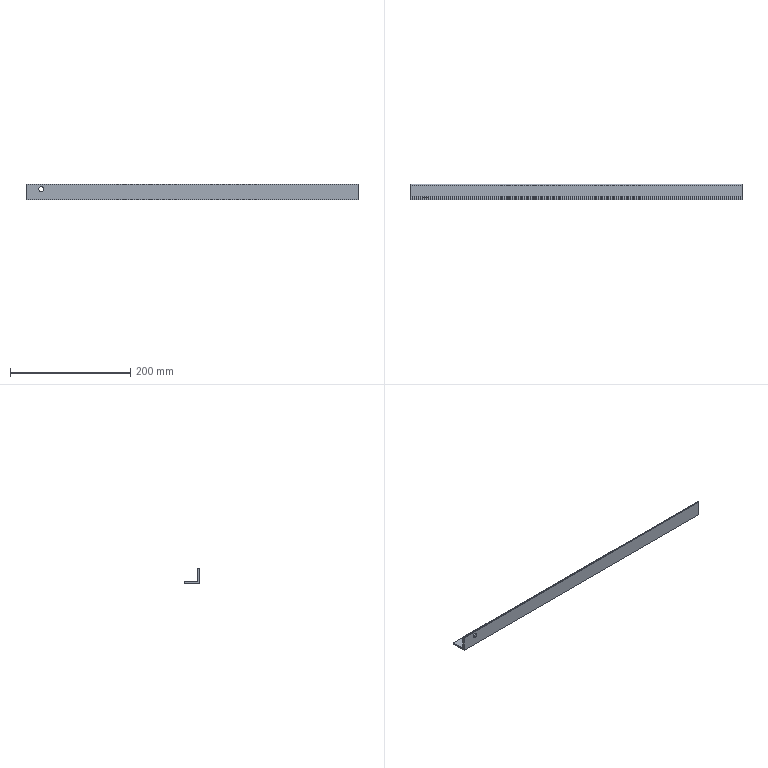Part | NX | features BREP 1 | 1 solid | 13 faces | box 552.45 x 25.4 x 25.4 mm | volume 83062 mm3 | plane 8 | cylinder 5 | commonest cylinder face diameters 3.175 x3 8.382 x2
STEP:
#1=CARTESIAN_POINT('',(-276.225,1.587,25.4));
#2=VERTEX_POINT('',#1);
#3=CARTESIAN_POINT('',(-276.225,3.175,23.812));
#4=VERTEX_POINT('',#3);
#5=CARTESIAN_POINT('',(-276.225,1.587,23.812));
#6=DIRECTION('',(-1.,0.,0.));
#7=DIRECTION('',(0.,0.,1.));
#8=AXIS2_PLACEMENT_3D('',#5,#6,#7);
#9=CIRCLE('',#8,1.587);
#10=EDGE_CURVE('',#2,#4,#9,.T.);
#11=ORIENTED_EDGE('',*,*,#10,.T.);
#12=CARTESIAN_POINT('',(-276.225,3.175,4.763));
#13=VERTEX_POINT('',#12);
#14=CARTESIAN_POINT('',(-276.225,3.175,4.763));
#15=DIRECTION('',(0.,0.,1.));
#16=VECTOR('',#15,1000.);
#17=LINE('',#14,#16);
#18=EDGE_CURVE('',#13,#4,#17,.T.);
#19=ORIENTED_EDGE('',*,*,#18,.F.);
#20=CARTESIAN_POINT('',(-276.225,4.763,3.175));
#21=VERTEX_POINT('',#20);
#22=CARTESIAN_POINT('',(-276.225,4.763,4.763));
#23=DIRECTION('',(1.,0.,0.));
#24=DIRECTION('',(0.,-1.,0.));
#25=AXIS2_PLACEMENT_3D('',#22,#23,#24);
#26=CIRCLE('',#25,1.587);
#27=EDGE_CURVE('',#13,#21,#26,.T.);
#28=ORIENTED_EDGE('',*,*,#27,.T.);
#29=CARTESIAN_POINT('',(-276.225,23.812,3.175));
#30=VERTEX_POINT('',#29);
#31=CARTESIAN_POINT('',(-276.225,23.812,3.175));
#32=DIRECTION('',(0.,-1.,0.));
#33=VECTOR('',#32,1000.);
#34=LINE('',#31,#33);
#35=EDGE_CURVE('',#30,#21,#34,.T.);
#36=ORIENTED_EDGE('',*,*,#35,.F.);
#37=CARTESIAN_POINT('',(-276.225,25.4,1.587));
#38=VERTEX_POINT('',#37);
#39=CARTESIAN_POINT('',(-276.225,23.812,1.587));
#40=DIRECTION('',(-1.,0.,0.));
#41=DIRECTION('',(0.,0.,1.));
#42=AXIS2_PLACEMENT_3D('',#39,#40,#41);
#43=CIRCLE('',#42,1.587);
#44=EDGE_CURVE('',#30,#38,#43,.T.);
#45=ORIENTED_EDGE('',*,*,#44,.T.);
#46=CARTESIAN_POINT('',(-276.225,25.4,0.));
#47=VERTEX_POINT('',#46);
#48=CARTESIAN_POINT('',(-276.225,25.4,0.));
#49=DIRECTION('',(0.,0.,1.));
#50=VECTOR('',#49,1000.);
#51=LINE('',#48,#50);
#52=EDGE_CURVE('',#47,#38,#51,.T.);
#53=ORIENTED_EDGE('',*,*,#52,.F.);
#54=CARTESIAN_POINT('',(-276.225,0.,0.));
#55=VERTEX_POINT('',#54);
#56=CARTESIAN_POINT('',(-276.225,0.,0.));
#57=DIRECTION('',(0.,1.,0.));
#58=VECTOR('',#57,1000.);
#59=LINE('',#56,#58);
#60=EDGE_CURVE('',#55,#47,#59,.T.);
#61=ORIENTED_EDGE('',*,*,#60,.F.);
#62=CARTESIAN_POINT('',(-276.225,0.,25.4));
#63=VERTEX_POINT('',#62);
#64=CARTESIAN_POINT('',(-276.225,0.,25.4));
#65=DIRECTION('',(0.,0.,-1.));
#66=VECTOR('',#65,1000.);
#67=LINE('',#64,#66);
#68=EDGE_CURVE('',#63,#55,#67,.T.);
#69=ORIENTED_EDGE('',*,*,#68,.F.);
#70=CARTESIAN_POINT('',(-276.225,1.587,25.4));
#71=DIRECTION('',(0.,-1.,0.));
#72=VECTOR('',#71,1000.);
#73=LINE('',#70,#72);
#74=EDGE_CURVE('',#2,#63,#73,.T.);
#75=ORIENTED_EDGE('',*,*,#74,.F.);
#76=EDGE_LOOP('',(#11,#19,#28,#36,#45,#53,#61,#69,#75));
#77=FACE_BOUND('',#76,.T.);
#78=CARTESIAN_POINT('',(-276.225,0.,0.));
#79=DIRECTION('',(1.,0.,0.));
#80=DIRECTION('',(0.,1.,0.));
#81=AXIS2_PLACEMENT_3D('',#78,#79,#80);
#82=PLANE('',#81);
#83=ADVANCED_FACE('',(#77),#82,.F.);
#84=CARTESIAN_POINT('',(276.225,0.,25.4));
#85=VERTEX_POINT('',#84);
#86=CARTESIAN_POINT('',(-276.225,0.,25.4));
#87=DIRECTION('',(1.,0.,0.));
#88=VECTOR('',#87,1000.);
#89=LINE('',#86,#88);
#90=EDGE_CURVE('',#63,#85,#89,.T.);
#91=ORIENTED_EDGE('',*,*,#90,.T.);
#92=CARTESIAN_POINT('',(276.225,1.587,25.4));
#93=VERTEX_POINT('',#92);
#94=CARTESIAN_POINT('',(276.225,1.587,25.4));
#95=DIRECTION('',(0.,-1.,0.));
#96=VECTOR('',#95,1000.);
#97=LINE('',#94,#96);
#98=EDGE_CURVE('',#93,#85,#97,.T.);
#99=ORIENTED_EDGE('',*,*,#98,.F.);
#100=CARTESIAN_POINT('',(276.225,1.587,25.4));
#101=DIRECTION('',(-1.,0.,0.));
#102=VECTOR('',#101,1000.);
#103=LINE('',#100,#102);
#104=EDGE_CURVE('',#93,#2,#103,.T.);
#105=ORIENTED_EDGE('',*,*,#104,.T.);
#106=ORIENTED_EDGE('',*,*,#74,.T.);
#107=EDGE_LOOP('',(#91,#99,#105,#106));
#108=FACE_BOUND('',#107,.T.);
#109=CARTESIAN_POINT('',(-276.225,3.175,25.4));
#110=DIRECTION('',(0.,0.,1.));
#111=DIRECTION('',(1.,0.,0.));
#112=AXIS2_PLACEMENT_3D('',#109,#110,#111);
#113=PLANE('',#112);
#114=ADVANCED_FACE('',(#108),#113,.T.);
#115=CARTESIAN_POINT('',(276.225,3.175,23.812));
#116=VERTEX_POINT('',#115);
#117=CARTESIAN_POINT('',(276.225,1.587,23.812));
#118=DIRECTION('',(1.,0.,0.));
#119=DIRECTION('',(0.,1.,0.));
#120=AXIS2_PLACEMENT_3D('',#117,#118,#119);
#121=CIRCLE('',#120,1.587);
#122=EDGE_CURVE('',#116,#93,#121,.T.);
#123=ORIENTED_EDGE('',*,*,#122,.F.);
#124=CARTESIAN_POINT('',(276.225,3.175,23.812));
#125=DIRECTION('',(-1.,0.,0.));
#126=VECTOR('',#125,1000.);
#127=LINE('',#124,#126);
#128=EDGE_CURVE('',#116,#4,#127,.T.);
#129=ORIENTED_EDGE('',*,*,#128,.T.);
#130=ORIENTED_EDGE('',*,*,#10,.F.);
#131=ORIENTED_EDGE('',*,*,#104,.F.);
#132=EDGE_LOOP('',(#123,#129,#130,#131));
#133=FACE_BOUND('',#132,.T.);
#134=CARTESIAN_POINT('',(277.091,1.587,23.812));
#135=DIRECTION('',(-1.,0.,0.));
#136=DIRECTION('',(0.,0.,1.));
#137=AXIS2_PLACEMENT_3D('',#134,#135,#136);
#138=CYLINDRICAL_SURFACE('',#137,1.587);
#139=ADVANCED_FACE('',(#133),#138,.T.);
#140=CARTESIAN_POINT('',(276.225,3.175,4.763));
#141=VERTEX_POINT('',#140);
#142=CARTESIAN_POINT('',(276.225,3.175,4.763));
#143=DIRECTION('',(0.,0.,1.));
#144=VECTOR('',#143,1000.);
#145=LINE('',#142,#144);
#146=EDGE_CURVE('',#141,#116,#145,.T.);
#147=ORIENTED_EDGE('',*,*,#146,.F.);
#148=CARTESIAN_POINT('',(-276.225,3.175,4.763));
#149=DIRECTION('',(1.,0.,0.));
#150=VECTOR('',#149,1000.);
#151=LINE('',#148,#150);
#152=EDGE_CURVE('',#13,#141,#151,.T.);
#153=ORIENTED_EDGE('',*,*,#152,.F.);
#154=ORIENTED_EDGE('',*,*,#18,.T.);
#155=ORIENTED_EDGE('',*,*,#128,.F.);
#156=EDGE_LOOP('',(#147,#153,#154,#155));
#157=FACE_BOUND('',#156,.T.);
#158=CARTESIAN_POINT('',(-255.016,3.175,17.475));
#159=VERTEX_POINT('',#158);
#160=CARTESIAN_POINT('',(-246.634,3.175,17.475));
#161=VERTEX_POINT('',#160);
#162=CARTESIAN_POINT('',(-250.825,3.175,17.475));
#163=DIRECTION('',(0.,-1.,0.));
#164=DIRECTION('',(-1.,0.,0.));
#165=AXIS2_PLACEMENT_3D('',#162,#163,#164);
#166=CIRCLE('',#165,4.191);
#167=EDGE_CURVE('',#159,#161,#166,.T.);
#168=ORIENTED_EDGE('',*,*,#167,.T.);
#169=CARTESIAN_POINT('',(-250.825,3.175,17.475));
#170=DIRECTION('',(0.,-1.,0.));
#171=DIRECTION('',(1.,0.,0.));
#172=AXIS2_PLACEMENT_3D('',#169,#170,#171);
#173=CIRCLE('',#172,4.191);
#174=EDGE_CURVE('',#161,#159,#173,.T.);
#175=ORIENTED_EDGE('',*,*,#174,.T.);
#176=EDGE_LOOP('',(#168,#175));
#177=FACE_BOUND('',#176,.T.);
#178=CARTESIAN_POINT('',(-276.225,3.175,3.175));
#179=DIRECTION('',(0.,1.,0.));
#180=DIRECTION('',(1.,0.,0.));
#181=AXIS2_PLACEMENT_3D('',#178,#179,#180);
#182=PLANE('',#181);
#183=ADVANCED_FACE('',(#157,#177),#182,.T.);
#184=CARTESIAN_POINT('',(276.225,4.763,3.175));
#185=VERTEX_POINT('',#184);
#186=CARTESIAN_POINT('',(276.225,4.763,4.763));
#187=DIRECTION('',(-1.,0.,0.));
#188=DIRECTION('',(0.,0.,-1.));
#189=AXIS2_PLACEMENT_3D('',#186,#187,#188);
#190=CIRCLE('',#189,1.587);
#191=EDGE_CURVE('',#185,#141,#190,.T.);
#192=ORIENTED_EDGE('',*,*,#191,.F.);
#193=CARTESIAN_POINT('',(-276.225,4.763,3.175));
#194=DIRECTION('',(1.,0.,0.));
#195=VECTOR('',#194,1000.);
#196=LINE('',#193,#195);
#197=EDGE_CURVE('',#21,#185,#196,.T.);
#198=ORIENTED_EDGE('',*,*,#197,.F.);
#199=ORIENTED_EDGE('',*,*,#27,.F.);
#200=ORIENTED_EDGE('',*,*,#152,.T.);
#201=EDGE_LOOP('',(#192,#198,#199,#200));
#202=FACE_BOUND('',#201,.T.);
#203=CARTESIAN_POINT('',(-276.965,4.763,4.763));
#204=DIRECTION('',(1.,0.,0.));
#205=DIRECTION('',(0.,-1.,0.));
#206=AXIS2_PLACEMENT_3D('',#203,#204,#205);
#207=CYLINDRICAL_SURFACE('',#206,1.587);
#208=ADVANCED_FACE('',(#202),#207,.F.);
#209=ORIENTED_EDGE('',*,*,#35,.T.);
#210=ORIENTED_EDGE('',*,*,#197,.T.);
#211=CARTESIAN_POINT('',(276.225,23.812,3.175));
#212=VERTEX_POINT('',#211);
#213=CARTESIAN_POINT('',(276.225,23.812,3.175));
#214=DIRECTION('',(0.,-1.,0.));
#215=VECTOR('',#214,1000.);
#216=LINE('',#213,#215);
#217=EDGE_CURVE('',#212,#185,#216,.T.);
#218=ORIENTED_EDGE('',*,*,#217,.F.);
#219=CARTESIAN_POINT('',(276.225,23.812,3.175));
#220=DIRECTION('',(-1.,0.,0.));
#221=VECTOR('',#220,1000.);
#222=LINE('',#219,#221);
#223=EDGE_CURVE('',#212,#30,#222,.T.);
#224=ORIENTED_EDGE('',*,*,#223,.T.);
#225=EDGE_LOOP('',(#209,#210,#218,#224));
#226=FACE_BOUND('',#225,.T.);
#227=CARTESIAN_POINT('',(-276.225,25.4,3.175));
#228=DIRECTION('',(0.,0.,1.));
#229=DIRECTION('',(1.,0.,0.));
#230=AXIS2_PLACEMENT_3D('',#227,#228,#229);
#231=PLANE('',#230);
#232=ADVANCED_FACE('',(#226),#231,.T.);
#233=CARTESIAN_POINT('',(276.225,25.4,1.587));
#234=VERTEX_POINT('',#233);
#235=CARTESIAN_POINT('',(276.225,23.812,1.587));
#236=DIRECTION('',(1.,0.,0.));
#237=DIRECTION('',(0.,1.,0.));
#238=AXIS2_PLACEMENT_3D('',#235,#236,#237);
#239=CIRCLE('',#238,1.587);
#240=EDGE_CURVE('',#234,#212,#239,.T.);
#241=ORIENTED_EDGE('',*,*,#240,.F.);
#242=CARTESIAN_POINT('',(276.225,25.4,1.587));
#243=DIRECTION('',(-1.,0.,0.));
#244=VECTOR('',#243,1000.);
#245=LINE('',#242,#244);
#246=EDGE_CURVE('',#234,#38,#245,.T.);
#247=ORIENTED_EDGE('',*,*,#246,.T.);
#248=ORIENTED_EDGE('',*,*,#44,.F.);
#249=ORIENTED_EDGE('',*,*,#223,.F.);
#250=EDGE_LOOP('',(#241,#247,#248,#249));
#251=FACE_BOUND('',#250,.T.);
#252=CARTESIAN_POINT('',(277.091,23.812,1.587));
#253=DIRECTION('',(-1.,0.,0.));
#254=DIRECTION('',(0.,0.,1.));
#255=AXIS2_PLACEMENT_3D('',#252,#253,#254);
#256=CYLINDRICAL_SURFACE('',#255,1.587);
#257=ADVANCED_FACE('',(#251),#256,.T.);
#258=ORIENTED_EDGE('',*,*,#246,.F.);
#259=CARTESIAN_POINT('',(276.225,25.4,0.));
#260=VERTEX_POINT('',#259);
#261=CARTESIAN_POINT('',(276.225,25.4,0.));
#262=DIRECTION('',(0.,0.,1.));
#263=VECTOR('',#262,1000.);
#264=LINE('',#261,#263);
#265=EDGE_CURVE('',#260,#234,#264,.T.);
#266=ORIENTED_EDGE('',*,*,#265,.F.);
#267=CARTESIAN_POINT('',(-276.225,25.4,0.));
#268=DIRECTION('',(1.,0.,0.));
#269=VECTOR('',#268,1000.);
#270=LINE('',#267,#269);
#271=EDGE_CURVE('',#47,#260,#270,.T.);
#272=ORIENTED_EDGE('',*,*,#271,.F.);
#273=ORIENTED_EDGE('',*,*,#52,.T.);
#274=EDGE_LOOP('',(#258,#266,#272,#273));
#275=FACE_BOUND('',#274,.T.);
#276=CARTESIAN_POINT('',(-276.225,25.4,0.));
#277=DIRECTION('',(0.,1.,0.));
#278=DIRECTION('',(1.,0.,0.));
#279=AXIS2_PLACEMENT_3D('',#276,#277,#278);
#280=PLANE('',#279);
#281=ADVANCED_FACE('',(#275),#280,.T.);
#282=ORIENTED_EDGE('',*,*,#271,.T.);
#283=CARTESIAN_POINT('',(276.225,0.,0.));
#284=VERTEX_POINT('',#283);
#285=CARTESIAN_POINT('',(276.225,0.,0.));
#286=DIRECTION('',(0.,1.,0.));
#287=VECTOR('',#286,1000.);
#288=LINE('',#285,#287);
#289=EDGE_CURVE('',#284,#260,#288,.T.);
#290=ORIENTED_EDGE('',*,*,#289,.F.);
#291=CARTESIAN_POINT('',(-276.225,0.,0.));
#292=DIRECTION('',(1.,0.,0.));
#293=VECTOR('',#292,1000.);
#294=LINE('',#291,#293);
#295=EDGE_CURVE('',#55,#284,#294,.T.);
#296=ORIENTED_EDGE('',*,*,#295,.F.);
#297=ORIENTED_EDGE('',*,*,#60,.T.);
#298=EDGE_LOOP('',(#282,#290,#296,#297));
#299=FACE_BOUND('',#298,.T.);
#300=CARTESIAN_POINT('',(-276.225,0.,0.));
#301=DIRECTION('',(0.,0.,-1.));
#302=DIRECTION('',(0.,-1.,0.));
#303=AXIS2_PLACEMENT_3D('',#300,#301,#302);
#304=PLANE('',#303);
#305=ADVANCED_FACE('',(#299),#304,.T.);
#306=ORIENTED_EDGE('',*,*,#295,.T.);
#307=CARTESIAN_POINT('',(276.225,0.,25.4));
#308=DIRECTION('',(0.,0.,-1.));
#309=VECTOR('',#308,1000.);
#310=LINE('',#307,#309);
#311=EDGE_CURVE('',#85,#284,#310,.T.);
#312=ORIENTED_EDGE('',*,*,#311,.F.);
#313=ORIENTED_EDGE('',*,*,#90,.F.);
#314=ORIENTED_EDGE('',*,*,#68,.T.);
#315=EDGE_LOOP('',(#306,#312,#313,#314));
#316=FACE_BOUND('',#315,.T.);
#317=CARTESIAN_POINT('',(-255.016,0.,17.475));
#318=VERTEX_POINT('',#317);
#319=CARTESIAN_POINT('',(-246.634,0.,17.475));
#320=VERTEX_POINT('',#319);
#321=CARTESIAN_POINT('',(-250.825,0.,17.475));
#322=DIRECTION('',(0.,-1.,0.));
#323=DIRECTION('',(-1.,0.,0.));
#324=AXIS2_PLACEMENT_3D('',#321,#322,#323);
#325=CIRCLE('',#324,4.191);
#326=EDGE_CURVE('',#318,#320,#325,.T.);
#327=ORIENTED_EDGE('',*,*,#326,.F.);
#328=CARTESIAN_POINT('',(-250.825,0.,17.475));
#329=DIRECTION('',(0.,-1.,0.));
#330=DIRECTION('',(1.,0.,0.));
#331=AXIS2_PLACEMENT_3D('',#328,#329,#330);
#332=CIRCLE('',#331,4.191);
#333=EDGE_CURVE('',#320,#318,#332,.T.);
#334=ORIENTED_EDGE('',*,*,#333,.F.);
#335=EDGE_LOOP('',(#327,#334));
#336=FACE_BOUND('',#335,.T.);
#337=CARTESIAN_POINT('',(-276.225,0.,25.4));
#338=DIRECTION('',(0.,-1.,0.));
#339=DIRECTION('',(0.,0.,-1.));
#340=AXIS2_PLACEMENT_3D('',#337,#338,#339);
#341=PLANE('',#340);
#342=ADVANCED_FACE('',(#316,#336),#341,.T.);
#343=ORIENTED_EDGE('',*,*,#311,.T.);
#344=ORIENTED_EDGE('',*,*,#289,.T.);
#345=ORIENTED_EDGE('',*,*,#265,.T.);
#346=ORIENTED_EDGE('',*,*,#240,.T.);
#347=ORIENTED_EDGE('',*,*,#217,.T.);
#348=ORIENTED_EDGE('',*,*,#191,.T.);
#349=ORIENTED_EDGE('',*,*,#146,.T.);
#350=ORIENTED_EDGE('',*,*,#122,.T.);
#351=ORIENTED_EDGE('',*,*,#98,.T.);
#352=EDGE_LOOP('',(#343,#344,#345,#346,#347,#348,#349,#350,#351));
#353=FACE_BOUND('',#352,.T.);
#354=CARTESIAN_POINT('',(276.225,0.,0.));
#355=DIRECTION('',(1.,0.,0.));
#356=DIRECTION('',(0.,1.,0.));
#357=AXIS2_PLACEMENT_3D('',#354,#355,#356);
#358=PLANE('',#357);
#359=ADVANCED_FACE('',(#353),#358,.T.);
#360=CARTESIAN_POINT('',(-246.634,3.175,17.475));
#361=DIRECTION('',(0.,-1.,0.));
#362=VECTOR('',#361,1000.);
#363=LINE('',#360,#362);
#364=EDGE_CURVE('',#320,#161,#363,.F.);
#365=ORIENTED_EDGE('',*,*,#364,.F.);
#366=ORIENTED_EDGE('',*,*,#333,.T.);
#367=CARTESIAN_POINT('',(-255.016,3.175,17.475));
#368=DIRECTION('',(0.,-1.,0.));
#369=VECTOR('',#368,1000.);
#370=LINE('',#367,#369);
#371=EDGE_CURVE('',#318,#159,#370,.F.);
#372=ORIENTED_EDGE('',*,*,#371,.T.);
#373=ORIENTED_EDGE('',*,*,#174,.F.);
#374=EDGE_LOOP('',(#365,#366,#372,#373));
#375=FACE_BOUND('',#374,.T.);
#376=CARTESIAN_POINT('',(-250.825,3.175,17.475));
#377=DIRECTION('',(0.,-1.,0.));
#378=DIRECTION('',(1.,0.,0.));
#379=AXIS2_PLACEMENT_3D('',#376,#377,#378);
#380=CYLINDRICAL_SURFACE('',#379,4.191);
#381=ADVANCED_FACE('',(#375),#380,.F.);
#382=ORIENTED_EDGE('',*,*,#371,.F.);
#383=ORIENTED_EDGE('',*,*,#326,.T.);
#384=ORIENTED_EDGE('',*,*,#364,.T.);
#385=ORIENTED_EDGE('',*,*,#167,.F.);
#386=EDGE_LOOP('',(#382,#383,#384,#385));
#387=FACE_BOUND('',#386,.T.);
#388=CARTESIAN_POINT('',(-250.825,3.175,17.475));
#389=DIRECTION('',(0.,-1.,0.));
#390=DIRECTION('',(1.,0.,0.));
#391=AXIS2_PLACEMENT_3D('',#388,#389,#390);
#392=CYLINDRICAL_SURFACE('',#391,4.191);
#393=ADVANCED_FACE('',(#387),#392,.F.);
#394=CLOSED_SHELL('',(#83,#114,#139,#183,#208,#232,#257,#281,#305,#342,#359,#381,#393));
#395=MANIFOLD_SOLID_BREP('',#394);
#396=(LENGTH_UNIT()NAMED_UNIT(*)SI_UNIT(.MILLI.,.METRE.));
#397=UNCERTAINTY_MEASURE_WITH_UNIT(LENGTH_MEASURE(0.00001),#396,'','');
#398=(NAMED_UNIT(*)PLANE_ANGLE_UNIT()SI_UNIT($,.RADIAN.));
#399=(NAMED_UNIT(*)SI_UNIT($,.STERADIAN.)SOLID_ANGLE_UNIT());
#400=(GEOMETRIC_REPRESENTATION_CONTEXT(3)GLOBAL_UNCERTAINTY_ASSIGNED_CONTEXT((#397))GLOBAL_UNIT_ASSIGNED_CONTEXT((#396,#398,#399))REPRESENTATION_CONTEXT('',''));
#401=ADVANCED_BREP_SHAPE_REPRESENTATION('',(#395),#400);